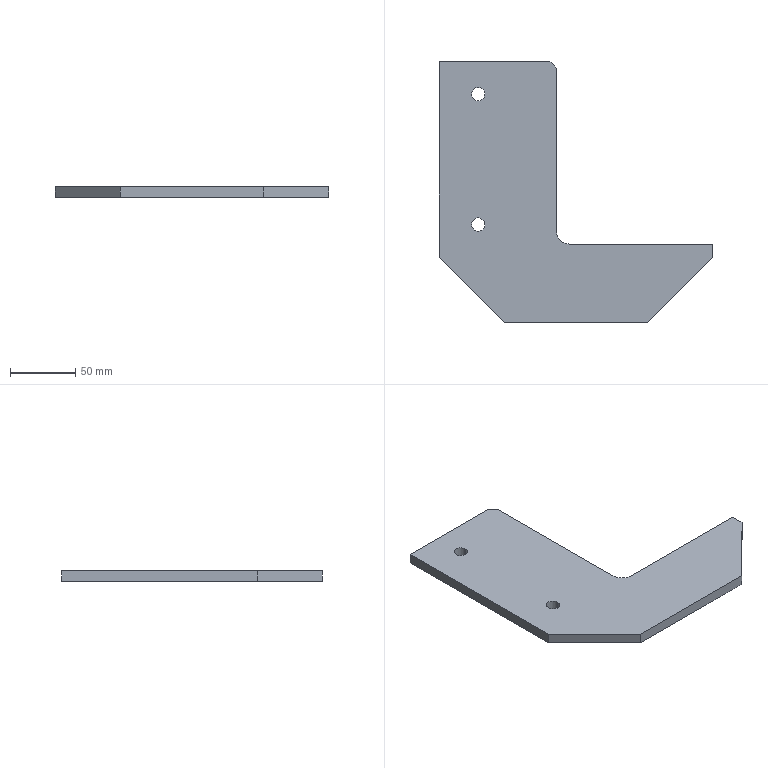Part | SolidWorks | features Chamfer 2, Extrusion 1, Fillet 1, HoleWzd 1, ICE 1 | 1 solid | 16 faces | box 210 x 200 x 8 mm | volume 180364 mm3 | plane 11 | cylinder 5 | commonest cylinder face diameters 10.2 x4 20 x1
STEP:
#1=CARTESIAN_POINT('',(-69.9,75.01,0.));
#2=VERTEX_POINT('',#1);
#3=CARTESIAN_POINT('',(-80.1,75.01,0.));
#4=VERTEX_POINT('',#3);
#5=CARTESIAN_POINT('',(-75.,75.01,0.));
#6=DIRECTION('',(0.,0.,-1.));
#7=DIRECTION('',(-1.,0.,0.));
#8=AXIS2_PLACEMENT_3D('',#5,#6,#7);
#9=CIRCLE('',#8,5.1);
#10=EDGE_CURVE('',#2,#4,#9,.T.);
#11=ORIENTED_EDGE('',*,*,#10,.T.);
#12=CARTESIAN_POINT('',(-80.1,75.01,8.));
#13=VERTEX_POINT('',#12);
#14=CARTESIAN_POINT('',(-80.1,75.01,8.));
#15=DIRECTION('',(0.,0.,1.));
#16=VECTOR('',#15,1000.);
#17=LINE('',#14,#16);
#18=EDGE_CURVE('',#4,#13,#17,.T.);
#19=ORIENTED_EDGE('',*,*,#18,.T.);
#20=CARTESIAN_POINT('',(-69.9,75.01,8.));
#21=VERTEX_POINT('',#20);
#22=CARTESIAN_POINT('',(-75.,75.01,8.));
#23=DIRECTION('',(0.,0.,1.));
#24=DIRECTION('',(1.,0.,0.));
#25=AXIS2_PLACEMENT_3D('',#22,#23,#24);
#26=CIRCLE('',#25,5.1);
#27=EDGE_CURVE('',#13,#21,#26,.T.);
#28=ORIENTED_EDGE('',*,*,#27,.T.);
#29=CARTESIAN_POINT('',(-69.9,75.01,8.));
#30=DIRECTION('',(0.,0.,1.));
#31=VECTOR('',#30,1000.);
#32=LINE('',#29,#31);
#33=EDGE_CURVE('',#2,#21,#32,.T.);
#34=ORIENTED_EDGE('',*,*,#33,.F.);
#35=EDGE_LOOP('',(#11,#19,#28,#34));
#36=FACE_OUTER_BOUND('',#35,.T.);
#37=CARTESIAN_POINT('',(-75.,75.01,8.));
#38=DIRECTION('',(0.,0.,1.));
#39=DIRECTION('',(1.,0.,0.));
#40=AXIS2_PLACEMENT_3D('',#37,#38,#39);
#41=CYLINDRICAL_SURFACE('',#40,5.1);
#42=ADVANCED_FACE('',(#36),#41,.F.);
#43=CARTESIAN_POINT('',(-69.9,-24.99,0.));
#44=VERTEX_POINT('',#43);
#45=CARTESIAN_POINT('',(-80.1,-24.99,0.));
#46=VERTEX_POINT('',#45);
#47=CARTESIAN_POINT('',(-75.,-24.99,0.));
#48=DIRECTION('',(0.,0.,-1.));
#49=DIRECTION('',(-1.,0.,0.));
#50=AXIS2_PLACEMENT_3D('',#47,#48,#49);
#51=CIRCLE('',#50,5.1);
#52=EDGE_CURVE('',#44,#46,#51,.T.);
#53=ORIENTED_EDGE('',*,*,#52,.T.);
#54=CARTESIAN_POINT('',(-80.1,-24.99,8.));
#55=VERTEX_POINT('',#54);
#56=CARTESIAN_POINT('',(-80.1,-24.99,8.));
#57=DIRECTION('',(0.,0.,1.));
#58=VECTOR('',#57,1000.);
#59=LINE('',#56,#58);
#60=EDGE_CURVE('',#46,#55,#59,.T.);
#61=ORIENTED_EDGE('',*,*,#60,.T.);
#62=CARTESIAN_POINT('',(-69.9,-24.99,8.));
#63=VERTEX_POINT('',#62);
#64=CARTESIAN_POINT('',(-75.,-24.99,8.));
#65=DIRECTION('',(0.,0.,1.));
#66=DIRECTION('',(1.,0.,0.));
#67=AXIS2_PLACEMENT_3D('',#64,#65,#66);
#68=CIRCLE('',#67,5.1);
#69=EDGE_CURVE('',#55,#63,#68,.T.);
#70=ORIENTED_EDGE('',*,*,#69,.T.);
#71=CARTESIAN_POINT('',(-69.9,-24.99,8.));
#72=DIRECTION('',(0.,0.,1.));
#73=VECTOR('',#72,1000.);
#74=LINE('',#71,#73);
#75=EDGE_CURVE('',#44,#63,#74,.T.);
#76=ORIENTED_EDGE('',*,*,#75,.F.);
#77=EDGE_LOOP('',(#53,#61,#70,#76));
#78=FACE_OUTER_BOUND('',#77,.T.);
#79=CARTESIAN_POINT('',(-75.,-24.99,8.));
#80=DIRECTION('',(0.,0.,1.));
#81=DIRECTION('',(1.,0.,0.));
#82=AXIS2_PLACEMENT_3D('',#79,#80,#81);
#83=CYLINDRICAL_SURFACE('',#82,5.1);
#84=ADVANCED_FACE('',(#78),#83,.F.);
#85=CARTESIAN_POINT('',(-105.,100.,0.));
#86=VERTEX_POINT('',#85);
#87=CARTESIAN_POINT('',(-105.,-50.,0.));
#88=VERTEX_POINT('',#87);
#89=CARTESIAN_POINT('',(-105.,100.,0.));
#90=DIRECTION('',(0.,-1.,0.));
#91=VECTOR('',#90,1000.);
#92=LINE('',#89,#91);
#93=EDGE_CURVE('',#86,#88,#92,.T.);
#94=ORIENTED_EDGE('',*,*,#93,.T.);
#95=CARTESIAN_POINT('',(-105.,-50.,8.));
#96=VERTEX_POINT('',#95);
#97=CARTESIAN_POINT('',(-105.,-50.,8.));
#98=DIRECTION('',(0.,0.,1.));
#99=VECTOR('',#98,1000.);
#100=LINE('',#97,#99);
#101=EDGE_CURVE('',#88,#96,#100,.T.);
#102=ORIENTED_EDGE('',*,*,#101,.T.);
#103=CARTESIAN_POINT('',(-105.,100.,8.));
#104=VERTEX_POINT('',#103);
#105=CARTESIAN_POINT('',(-105.,100.,8.));
#106=DIRECTION('',(0.,-1.,0.));
#107=VECTOR('',#106,1000.);
#108=LINE('',#105,#107);
#109=EDGE_CURVE('',#104,#96,#108,.T.);
#110=ORIENTED_EDGE('',*,*,#109,.F.);
#111=CARTESIAN_POINT('',(-105.,100.,8.));
#112=DIRECTION('',(0.,0.,-1.));
#113=VECTOR('',#112,1000.);
#114=LINE('',#111,#113);
#115=EDGE_CURVE('',#104,#86,#114,.T.);
#116=ORIENTED_EDGE('',*,*,#115,.T.);
#117=EDGE_LOOP('',(#94,#102,#110,#116));
#118=FACE_OUTER_BOUND('',#117,.T.);
#119=CARTESIAN_POINT('',(-105.,100.,8.));
#120=DIRECTION('',(1.,0.,0.));
#121=DIRECTION('',(0.,1.,0.));
#122=AXIS2_PLACEMENT_3D('',#119,#120,#121);
#123=PLANE('',#122);
#124=ADVANCED_FACE('',(#118),#123,.F.);
#125=CARTESIAN_POINT('',(-55.,-100.,0.));
#126=VERTEX_POINT('',#125);
#127=CARTESIAN_POINT('',(55.,-100.,0.));
#128=VERTEX_POINT('',#127);
#129=CARTESIAN_POINT('',(105.,-100.,0.));
#130=DIRECTION('',(1.,0.,0.));
#131=VECTOR('',#130,1000.);
#132=LINE('',#129,#131);
#133=EDGE_CURVE('',#126,#128,#132,.T.);
#134=ORIENTED_EDGE('',*,*,#133,.T.);
#135=CARTESIAN_POINT('',(55.,-100.,8.));
#136=VERTEX_POINT('',#135);
#137=CARTESIAN_POINT('',(55.,-100.,8.));
#138=DIRECTION('',(0.,0.,1.));
#139=VECTOR('',#138,1000.);
#140=LINE('',#137,#139);
#141=EDGE_CURVE('',#128,#136,#140,.T.);
#142=ORIENTED_EDGE('',*,*,#141,.T.);
#143=CARTESIAN_POINT('',(-55.,-100.,8.));
#144=VERTEX_POINT('',#143);
#145=CARTESIAN_POINT('',(105.,-100.,8.));
#146=DIRECTION('',(1.,0.,0.));
#147=VECTOR('',#146,1000.);
#148=LINE('',#145,#147);
#149=EDGE_CURVE('',#144,#136,#148,.T.);
#150=ORIENTED_EDGE('',*,*,#149,.F.);
#151=CARTESIAN_POINT('',(-55.,-100.,8.));
#152=DIRECTION('',(0.,0.,-1.));
#153=VECTOR('',#152,1000.);
#154=LINE('',#151,#153);
#155=EDGE_CURVE('',#144,#126,#154,.T.);
#156=ORIENTED_EDGE('',*,*,#155,.T.);
#157=EDGE_LOOP('',(#134,#142,#150,#156));
#158=FACE_OUTER_BOUND('',#157,.T.);
#159=CARTESIAN_POINT('',(105.,-100.,8.));
#160=DIRECTION('',(0.,1.,0.));
#161=DIRECTION('',(-1.,0.,0.));
#162=AXIS2_PLACEMENT_3D('',#159,#160,#161);
#163=PLANE('',#162);
#164=ADVANCED_FACE('',(#158),#163,.F.);
#165=CARTESIAN_POINT('',(105.,-50.,0.));
#166=VERTEX_POINT('',#165);
#167=CARTESIAN_POINT('',(105.,-40.,0.));
#168=VERTEX_POINT('',#167);
#169=CARTESIAN_POINT('',(105.,100.,0.));
#170=DIRECTION('',(0.,1.,0.));
#171=VECTOR('',#170,1000.);
#172=LINE('',#169,#171);
#173=EDGE_CURVE('',#166,#168,#172,.T.);
#174=ORIENTED_EDGE('',*,*,#173,.T.);
#175=CARTESIAN_POINT('',(105.,-40.,8.));
#176=VERTEX_POINT('',#175);
#177=CARTESIAN_POINT('',(105.,-40.,8.));
#178=DIRECTION('',(0.,0.,1.));
#179=VECTOR('',#178,1000.);
#180=LINE('',#177,#179);
#181=EDGE_CURVE('',#168,#176,#180,.T.);
#182=ORIENTED_EDGE('',*,*,#181,.T.);
#183=CARTESIAN_POINT('',(105.,-50.,8.));
#184=VERTEX_POINT('',#183);
#185=CARTESIAN_POINT('',(105.,100.,8.));
#186=DIRECTION('',(0.,1.,0.));
#187=VECTOR('',#186,1000.);
#188=LINE('',#185,#187);
#189=EDGE_CURVE('',#184,#176,#188,.T.);
#190=ORIENTED_EDGE('',*,*,#189,.F.);
#191=CARTESIAN_POINT('',(105.,-50.,8.));
#192=DIRECTION('',(0.,0.,-1.));
#193=VECTOR('',#192,1000.);
#194=LINE('',#191,#193);
#195=EDGE_CURVE('',#184,#166,#194,.T.);
#196=ORIENTED_EDGE('',*,*,#195,.T.);
#197=EDGE_LOOP('',(#174,#182,#190,#196));
#198=FACE_OUTER_BOUND('',#197,.T.);
#199=CARTESIAN_POINT('',(105.,100.,8.));
#200=DIRECTION('',(-1.,0.,0.));
#201=DIRECTION('',(0.,-1.,0.));
#202=AXIS2_PLACEMENT_3D('',#199,#200,#201);
#203=PLANE('',#202);
#204=ADVANCED_FACE('',(#198),#203,.F.);
#205=CARTESIAN_POINT('',(-20.,100.,8.));
#206=VERTEX_POINT('',#205);
#207=CARTESIAN_POINT('',(105.,100.,8.));
#208=DIRECTION('',(-1.,0.,0.));
#209=VECTOR('',#208,1000.);
#210=LINE('',#207,#209);
#211=EDGE_CURVE('',#206,#104,#210,.T.);
#212=ORIENTED_EDGE('',*,*,#211,.F.);
#213=CARTESIAN_POINT('',(-20.,100.,0.));
#214=VERTEX_POINT('',#213);
#215=CARTESIAN_POINT('',(-20.,100.,8.));
#216=DIRECTION('',(0.,0.,-1.));
#217=VECTOR('',#216,1000.);
#218=LINE('',#215,#217);
#219=EDGE_CURVE('',#206,#214,#218,.T.);
#220=ORIENTED_EDGE('',*,*,#219,.T.);
#221=CARTESIAN_POINT('',(105.,100.,0.));
#222=DIRECTION('',(-1.,0.,0.));
#223=VECTOR('',#222,1000.);
#224=LINE('',#221,#223);
#225=EDGE_CURVE('',#214,#86,#224,.T.);
#226=ORIENTED_EDGE('',*,*,#225,.T.);
#227=ORIENTED_EDGE('',*,*,#115,.F.);
#228=EDGE_LOOP('',(#212,#220,#226,#227));
#229=FACE_OUTER_BOUND('',#228,.T.);
#230=CARTESIAN_POINT('',(105.,100.,8.));
#231=DIRECTION('',(0.,-1.,0.));
#232=DIRECTION('',(1.,0.,0.));
#233=AXIS2_PLACEMENT_3D('',#230,#231,#232);
#234=PLANE('',#233);
#235=ADVANCED_FACE('',(#229),#234,.F.);
#236=CARTESIAN_POINT('',(-75.,75.01,8.));
#237=DIRECTION('',(0.,0.,1.));
#238=DIRECTION('',(1.,0.,0.));
#239=AXIS2_PLACEMENT_3D('',#236,#237,#238);
#240=CIRCLE('',#239,5.1);
#241=EDGE_CURVE('',#21,#13,#240,.T.);
#242=ORIENTED_EDGE('',*,*,#241,.F.);
#243=ORIENTED_EDGE('',*,*,#27,.F.);
#244=EDGE_LOOP('',(#242,#243));
#245=FACE_BOUND('',#244,.T.);
#246=CARTESIAN_POINT('',(-75.,-24.99,8.));
#247=DIRECTION('',(0.,0.,1.));
#248=DIRECTION('',(1.,0.,0.));
#249=AXIS2_PLACEMENT_3D('',#246,#247,#248);
#250=CIRCLE('',#249,5.1);
#251=EDGE_CURVE('',#63,#55,#250,.T.);
#252=ORIENTED_EDGE('',*,*,#251,.F.);
#253=ORIENTED_EDGE('',*,*,#69,.F.);
#254=EDGE_LOOP('',(#252,#253));
#255=FACE_BOUND('',#254,.T.);
#256=CARTESIAN_POINT('',(-15.,95.,8.));
#257=VERTEX_POINT('',#256);
#258=CARTESIAN_POINT('',(-15.,-30.,8.));
#259=VERTEX_POINT('',#258);
#260=CARTESIAN_POINT('',(-15.,-40.,8.));
#261=DIRECTION('',(0.,-1.,0.));
#262=VECTOR('',#261,1000.);
#263=LINE('',#260,#262);
#264=EDGE_CURVE('',#257,#259,#263,.T.);
#265=ORIENTED_EDGE('',*,*,#264,.F.);
#266=CARTESIAN_POINT('',(-20.,100.,8.));
#267=DIRECTION('',(-0.7071,0.7071,0.));
#268=VECTOR('',#267,1000.);
#269=LINE('',#266,#268);
#270=EDGE_CURVE('',#257,#206,#269,.T.);
#271=ORIENTED_EDGE('',*,*,#270,.T.);
#272=ORIENTED_EDGE('',*,*,#211,.T.);
#273=ORIENTED_EDGE('',*,*,#109,.T.);
#274=CARTESIAN_POINT('',(-55.,-100.,8.));
#275=DIRECTION('',(0.7071,-0.7071,0.));
#276=VECTOR('',#275,1000.);
#277=LINE('',#274,#276);
#278=EDGE_CURVE('',#96,#144,#277,.T.);
#279=ORIENTED_EDGE('',*,*,#278,.T.);
#280=ORIENTED_EDGE('',*,*,#149,.T.);
#281=CARTESIAN_POINT('',(105.,-50.,8.));
#282=DIRECTION('',(0.7071,0.7071,0.));
#283=VECTOR('',#282,1000.);
#284=LINE('',#281,#283);
#285=EDGE_CURVE('',#136,#184,#284,.T.);
#286=ORIENTED_EDGE('',*,*,#285,.T.);
#287=ORIENTED_EDGE('',*,*,#189,.T.);
#288=CARTESIAN_POINT('',(-5.,-40.,8.));
#289=VERTEX_POINT('',#288);
#290=CARTESIAN_POINT('',(-15.,-40.,8.));
#291=DIRECTION('',(1.,0.,0.));
#292=VECTOR('',#291,1000.);
#293=LINE('',#290,#292);
#294=EDGE_CURVE('',#289,#176,#293,.T.);
#295=ORIENTED_EDGE('',*,*,#294,.F.);
#296=CARTESIAN_POINT('',(-5.,-30.,8.));
#297=DIRECTION('',(0.,0.,-1.));
#298=DIRECTION('',(-1.,0.,0.));
#299=AXIS2_PLACEMENT_3D('',#296,#297,#298);
#300=CIRCLE('',#299,10.);
#301=EDGE_CURVE('',#289,#259,#300,.T.);
#302=ORIENTED_EDGE('',*,*,#301,.T.);
#303=EDGE_LOOP('',(#265,#271,#272,#273,#279,#280,#286,#287,#295,#302));
#304=FACE_OUTER_BOUND('',#303,.T.);
#305=CARTESIAN_POINT('',(0.,0.,8.));
#306=DIRECTION('',(0.,0.,-1.));
#307=DIRECTION('',(-1.,0.,0.));
#308=AXIS2_PLACEMENT_3D('',#305,#306,#307);
#309=PLANE('',#308);
#310=ADVANCED_FACE('',(#245,#255,#304),#309,.F.);
#311=ORIENTED_EDGE('',*,*,#225,.F.);
#312=CARTESIAN_POINT('',(-15.,95.,0.));
#313=VERTEX_POINT('',#312);
#314=CARTESIAN_POINT('',(40.,40.,0.));
#315=DIRECTION('',(0.7071,-0.7071,0.));
#316=VECTOR('',#315,1000.);
#317=LINE('',#314,#316);
#318=EDGE_CURVE('',#214,#313,#317,.T.);
#319=ORIENTED_EDGE('',*,*,#318,.T.);
#320=CARTESIAN_POINT('',(-15.,-30.,0.));
#321=VERTEX_POINT('',#320);
#322=CARTESIAN_POINT('',(-15.,0.,0.));
#323=DIRECTION('',(0.,1.,0.));
#324=VECTOR('',#323,1000.);
#325=LINE('',#322,#324);
#326=EDGE_CURVE('',#321,#313,#325,.T.);
#327=ORIENTED_EDGE('',*,*,#326,.F.);
#328=CARTESIAN_POINT('',(-5.,-40.,0.));
#329=VERTEX_POINT('',#328);
#330=CARTESIAN_POINT('',(-5.,-30.,0.));
#331=DIRECTION('',(0.,0.,1.));
#332=DIRECTION('',(-1.,0.,0.));
#333=AXIS2_PLACEMENT_3D('',#330,#331,#332);
#334=CIRCLE('',#333,10.);
#335=EDGE_CURVE('',#321,#329,#334,.T.);
#336=ORIENTED_EDGE('',*,*,#335,.T.);
#337=CARTESIAN_POINT('',(-15.,-40.,0.));
#338=DIRECTION('',(1.,0.,0.));
#339=VECTOR('',#338,1000.);
#340=LINE('',#337,#339);
#341=EDGE_CURVE('',#329,#168,#340,.T.);
#342=ORIENTED_EDGE('',*,*,#341,.T.);
#343=ORIENTED_EDGE('',*,*,#173,.F.);
#344=CARTESIAN_POINT('',(77.5,-77.5,0.));
#345=DIRECTION('',(-0.7071,-0.7071,0.));
#346=VECTOR('',#345,1000.);
#347=LINE('',#344,#346);
#348=EDGE_CURVE('',#166,#128,#347,.T.);
#349=ORIENTED_EDGE('',*,*,#348,.T.);
#350=ORIENTED_EDGE('',*,*,#133,.F.);
#351=CARTESIAN_POINT('',(-77.5,-77.5,0.));
#352=DIRECTION('',(-0.7071,0.7071,0.));
#353=VECTOR('',#352,1000.);
#354=LINE('',#351,#353);
#355=EDGE_CURVE('',#126,#88,#354,.T.);
#356=ORIENTED_EDGE('',*,*,#355,.T.);
#357=ORIENTED_EDGE('',*,*,#93,.F.);
#358=EDGE_LOOP('',(#311,#319,#327,#336,#342,#343,#349,#350,#356,#357));
#359=FACE_OUTER_BOUND('',#358,.T.);
#360=ORIENTED_EDGE('',*,*,#10,.F.);
#361=CARTESIAN_POINT('',(-75.,75.01,0.));
#362=DIRECTION('',(0.,0.,-1.));
#363=DIRECTION('',(-1.,0.,0.));
#364=AXIS2_PLACEMENT_3D('',#361,#362,#363);
#365=CIRCLE('',#364,5.1);
#366=EDGE_CURVE('',#4,#2,#365,.T.);
#367=ORIENTED_EDGE('',*,*,#366,.F.);
#368=EDGE_LOOP('',(#360,#367));
#369=FACE_BOUND('',#368,.T.);
#370=ORIENTED_EDGE('',*,*,#52,.F.);
#371=CARTESIAN_POINT('',(-75.,-24.99,0.));
#372=DIRECTION('',(0.,0.,-1.));
#373=DIRECTION('',(-1.,0.,0.));
#374=AXIS2_PLACEMENT_3D('',#371,#372,#373);
#375=CIRCLE('',#374,5.1);
#376=EDGE_CURVE('',#46,#44,#375,.T.);
#377=ORIENTED_EDGE('',*,*,#376,.F.);
#378=EDGE_LOOP('',(#370,#377));
#379=FACE_BOUND('',#378,.T.);
#380=CARTESIAN_POINT('',(0.,0.,0.));
#381=DIRECTION('',(0.,0.,-1.));
#382=DIRECTION('',(-1.,0.,0.));
#383=AXIS2_PLACEMENT_3D('',#380,#381,#382);
#384=PLANE('',#383);
#385=ADVANCED_FACE('',(#359,#369,#379),#384,.T.);
#386=ORIENTED_EDGE('',*,*,#285,.F.);
#387=ORIENTED_EDGE('',*,*,#141,.F.);
#388=ORIENTED_EDGE('',*,*,#348,.F.);
#389=ORIENTED_EDGE('',*,*,#195,.F.);
#390=EDGE_LOOP('',(#386,#387,#388,#389));
#391=FACE_OUTER_BOUND('',#390,.T.);
#392=CARTESIAN_POINT('',(105.,-50.,8.));
#393=DIRECTION('',(-0.7071,0.7071,0.));
#394=DIRECTION('',(0.,0.,-1.));
#395=AXIS2_PLACEMENT_3D('',#392,#393,#394);
#396=PLANE('',#395);
#397=ADVANCED_FACE('',(#391),#396,.F.);
#398=ORIENTED_EDGE('',*,*,#278,.F.);
#399=ORIENTED_EDGE('',*,*,#101,.F.);
#400=ORIENTED_EDGE('',*,*,#355,.F.);
#401=ORIENTED_EDGE('',*,*,#155,.F.);
#402=EDGE_LOOP('',(#398,#399,#400,#401));
#403=FACE_OUTER_BOUND('',#402,.T.);
#404=CARTESIAN_POINT('',(-55.,-100.,8.));
#405=DIRECTION('',(0.7071,0.7071,0.));
#406=DIRECTION('',(0.,0.,-1.));
#407=AXIS2_PLACEMENT_3D('',#404,#405,#406);
#408=PLANE('',#407);
#409=ADVANCED_FACE('',(#403),#408,.F.);
#410=ORIENTED_EDGE('',*,*,#60,.F.);
#411=ORIENTED_EDGE('',*,*,#376,.T.);
#412=ORIENTED_EDGE('',*,*,#75,.T.);
#413=ORIENTED_EDGE('',*,*,#251,.T.);
#414=EDGE_LOOP('',(#410,#411,#412,#413));
#415=FACE_OUTER_BOUND('',#414,.T.);
#416=CARTESIAN_POINT('',(-75.,-24.99,8.));
#417=DIRECTION('',(0.,0.,1.));
#418=DIRECTION('',(1.,0.,0.));
#419=AXIS2_PLACEMENT_3D('',#416,#417,#418);
#420=CYLINDRICAL_SURFACE('',#419,5.1);
#421=ADVANCED_FACE('',(#415),#420,.F.);
#422=ORIENTED_EDGE('',*,*,#18,.F.);
#423=ORIENTED_EDGE('',*,*,#366,.T.);
#424=ORIENTED_EDGE('',*,*,#33,.T.);
#425=ORIENTED_EDGE('',*,*,#241,.T.);
#426=EDGE_LOOP('',(#422,#423,#424,#425));
#427=FACE_OUTER_BOUND('',#426,.T.);
#428=CARTESIAN_POINT('',(-75.,75.01,8.));
#429=DIRECTION('',(0.,0.,1.));
#430=DIRECTION('',(1.,0.,0.));
#431=AXIS2_PLACEMENT_3D('',#428,#429,#430);
#432=CYLINDRICAL_SURFACE('',#431,5.1);
#433=ADVANCED_FACE('',(#427),#432,.F.);
#434=ORIENTED_EDGE('',*,*,#341,.F.);
#435=CARTESIAN_POINT('',(-5.,-40.,8.));
#436=DIRECTION('',(0.,0.,1.));
#437=VECTOR('',#436,1000.);
#438=LINE('',#435,#437);
#439=EDGE_CURVE('',#329,#289,#438,.T.);
#440=ORIENTED_EDGE('',*,*,#439,.T.);
#441=ORIENTED_EDGE('',*,*,#294,.T.);
#442=ORIENTED_EDGE('',*,*,#181,.F.);
#443=EDGE_LOOP('',(#434,#440,#441,#442));
#444=FACE_OUTER_BOUND('',#443,.T.);
#445=CARTESIAN_POINT('',(-15.,-40.,0.));
#446=DIRECTION('',(0.,-1.,0.));
#447=DIRECTION('',(0.,0.,-1.));
#448=AXIS2_PLACEMENT_3D('',#445,#446,#447);
#449=PLANE('',#448);
#450=ADVANCED_FACE('',(#444),#449,.F.);
#451=ORIENTED_EDGE('',*,*,#264,.T.);
#452=CARTESIAN_POINT('',(-15.,-30.,0.));
#453=DIRECTION('',(0.,0.,-1.));
#454=VECTOR('',#453,1000.);
#455=LINE('',#452,#454);
#456=EDGE_CURVE('',#259,#321,#455,.T.);
#457=ORIENTED_EDGE('',*,*,#456,.T.);
#458=ORIENTED_EDGE('',*,*,#326,.T.);
#459=CARTESIAN_POINT('',(-15.,95.,0.));
#460=DIRECTION('',(0.,0.,1.));
#461=VECTOR('',#460,1000.);
#462=LINE('',#459,#461);
#463=EDGE_CURVE('',#313,#257,#462,.T.);
#464=ORIENTED_EDGE('',*,*,#463,.T.);
#465=EDGE_LOOP('',(#451,#457,#458,#464));
#466=FACE_OUTER_BOUND('',#465,.T.);
#467=CARTESIAN_POINT('',(-15.,-40.,0.));
#468=DIRECTION('',(-1.,0.,0.));
#469=DIRECTION('',(0.,0.,1.));
#470=AXIS2_PLACEMENT_3D('',#467,#468,#469);
#471=PLANE('',#470);
#472=ADVANCED_FACE('',(#466),#471,.F.);
#473=ORIENTED_EDGE('',*,*,#270,.F.);
#474=ORIENTED_EDGE('',*,*,#463,.F.);
#475=ORIENTED_EDGE('',*,*,#318,.F.);
#476=ORIENTED_EDGE('',*,*,#219,.F.);
#477=EDGE_LOOP('',(#473,#474,#475,#476));
#478=FACE_OUTER_BOUND('',#477,.T.);
#479=CARTESIAN_POINT('',(-20.,100.,8.));
#480=DIRECTION('',(-0.7071,-0.7071,0.));
#481=DIRECTION('',(0.,0.,-1.));
#482=AXIS2_PLACEMENT_3D('',#479,#480,#481);
#483=PLANE('',#482);
#484=ADVANCED_FACE('',(#478),#483,.F.);
#485=ORIENTED_EDGE('',*,*,#335,.F.);
#486=ORIENTED_EDGE('',*,*,#456,.F.);
#487=ORIENTED_EDGE('',*,*,#301,.F.);
#488=ORIENTED_EDGE('',*,*,#439,.F.);
#489=EDGE_LOOP('',(#485,#486,#487,#488));
#490=FACE_OUTER_BOUND('',#489,.T.);
#491=CARTESIAN_POINT('',(-5.,-30.,0.));
#492=DIRECTION('',(0.,0.,-1.));
#493=DIRECTION('',(-1.,0.,0.));
#494=AXIS2_PLACEMENT_3D('',#491,#492,#493);
#495=CYLINDRICAL_SURFACE('',#494,10.);
#496=ADVANCED_FACE('',(#490),#495,.F.);
#497=CLOSED_SHELL('',(#42,#84,#124,#164,#204,#235,#310,#385,#397,#409,#421,#433,#450,#472,#484,#496));
#498=MANIFOLD_SOLID_BREP('',#497);
#499=CARTESIAN_POINT('',(0.,0.,0.));
#500=DIRECTION('',(0.,0.,1.));
#501=DIRECTION('',(1.,0.,0.));
#502=AXIS2_PLACEMENT_3D('',#499,#500,#501);
#503=(LENGTH_UNIT()NAMED_UNIT(*)SI_UNIT(.MILLI.,.METRE.));
#504=UNCERTAINTY_MEASURE_WITH_UNIT(LENGTH_MEASURE(0.00001),#503,'','');
#505=(NAMED_UNIT(*)PLANE_ANGLE_UNIT()SI_UNIT($,.RADIAN.));
#506=(NAMED_UNIT(*)SI_UNIT($,.STERADIAN.)SOLID_ANGLE_UNIT());
#507=(GEOMETRIC_REPRESENTATION_CONTEXT(3)GLOBAL_UNCERTAINTY_ASSIGNED_CONTEXT((#504))GLOBAL_UNIT_ASSIGNED_CONTEXT((#503,#505,#506))REPRESENTATION_CONTEXT('',''));
#508=ADVANCED_BREP_SHAPE_REPRESENTATION('',(#498,#502),#507);